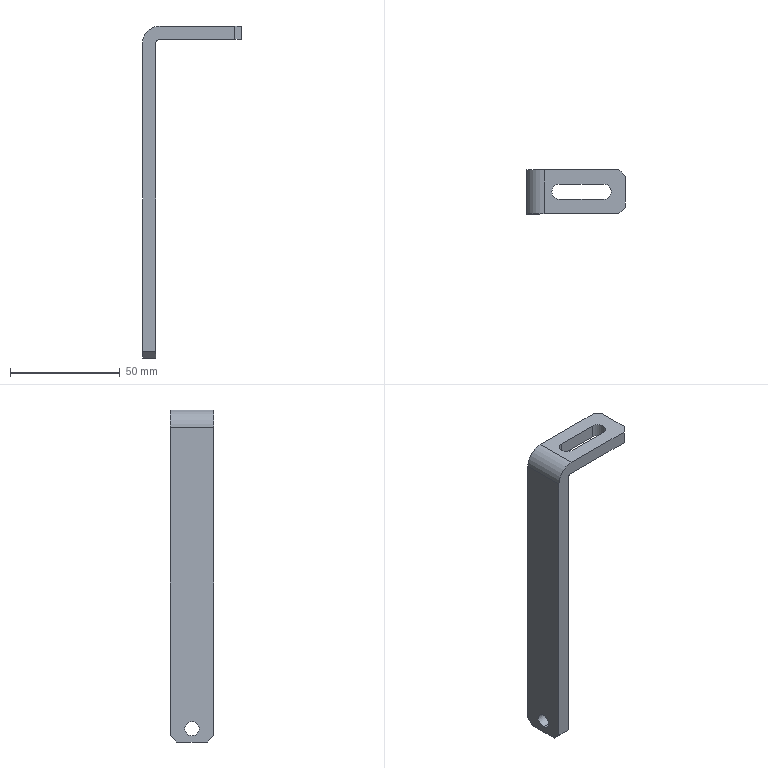Part | SolidWorks | features ICE 3, Fillet 2, Chamfer 1, Extrusion 1 | 1 solid | 21 faces | box 45 x 20 x 151 mm | volume 21164 mm3 | plane 14 | cylinder 7 | commonest cylinder face diameters 7 x3 6.5 x2 4 x1 16 x1
STEP:
#1=CARTESIAN_POINT('',(-11.,10.,75.5));
#2=VERTEX_POINT('',#1);
#3=CARTESIAN_POINT('',(-7.5,13.5,75.5));
#4=VERTEX_POINT('',#3);
#5=CARTESIAN_POINT('',(-7.5,10.,75.5));
#6=DIRECTION('',(0.,0.,-1.));
#7=DIRECTION('',(-1.,0.,0.));
#8=AXIS2_PLACEMENT_3D('',#5,#6,#7);
#9=CIRCLE('',#8,3.5);
#10=EDGE_CURVE('',#2,#4,#9,.T.);
#11=ORIENTED_EDGE('',*,*,#10,.F.);
#12=CARTESIAN_POINT('',(-11.,10.,69.5));
#13=VERTEX_POINT('',#12);
#14=CARTESIAN_POINT('',(-11.,10.,75.5));
#15=DIRECTION('',(0.,0.,-1.));
#16=VECTOR('',#15,1000.);
#17=LINE('',#14,#16);
#18=EDGE_CURVE('',#2,#13,#17,.T.);
#19=ORIENTED_EDGE('',*,*,#18,.T.);
#20=CARTESIAN_POINT('',(-7.5,13.5,69.5));
#21=VERTEX_POINT('',#20);
#22=CARTESIAN_POINT('',(-7.5,10.,69.5));
#23=DIRECTION('',(0.,0.,-1.));
#24=DIRECTION('',(-1.,0.,0.));
#25=AXIS2_PLACEMENT_3D('',#22,#23,#24);
#26=CIRCLE('',#25,3.5);
#27=EDGE_CURVE('',#13,#21,#26,.T.);
#28=ORIENTED_EDGE('',*,*,#27,.T.);
#29=CARTESIAN_POINT('',(-7.5,13.5,75.5));
#30=DIRECTION('',(0.,0.,-1.));
#31=VECTOR('',#30,1000.);
#32=LINE('',#29,#31);
#33=EDGE_CURVE('',#4,#21,#32,.T.);
#34=ORIENTED_EDGE('',*,*,#33,.F.);
#35=EDGE_LOOP('',(#11,#19,#28,#34));
#36=FACE_OUTER_BOUND('',#35,.T.);
#37=CARTESIAN_POINT('',(-7.5,10.,75.5));
#38=DIRECTION('',(0.,0.,-1.));
#39=DIRECTION('',(-1.,0.,0.));
#40=AXIS2_PLACEMENT_3D('',#37,#38,#39);
#41=CYLINDRICAL_SURFACE('',#40,3.5);
#42=ADVANCED_FACE('',(#36),#41,.F.);
#43=CARTESIAN_POINT('',(-22.5,10.,-66.25));
#44=VERTEX_POINT('',#43);
#45=CARTESIAN_POINT('',(-22.5,10.,-72.75));
#46=VERTEX_POINT('',#45);
#47=CARTESIAN_POINT('',(-22.5,10.,-69.5));
#48=DIRECTION('',(1.,0.,0.));
#49=DIRECTION('',(0.,0.,-1.));
#50=AXIS2_PLACEMENT_3D('',#47,#48,#49);
#51=CIRCLE('',#50,3.25);
#52=EDGE_CURVE('',#44,#46,#51,.T.);
#53=ORIENTED_EDGE('',*,*,#52,.F.);
#54=CARTESIAN_POINT('',(-16.5,10.,-66.25));
#55=VERTEX_POINT('',#54);
#56=CARTESIAN_POINT('',(-22.5,10.,-66.25));
#57=DIRECTION('',(1.,0.,0.));
#58=VECTOR('',#57,1000.);
#59=LINE('',#56,#58);
#60=EDGE_CURVE('',#44,#55,#59,.T.);
#61=ORIENTED_EDGE('',*,*,#60,.T.);
#62=CARTESIAN_POINT('',(-16.5,10.,-72.75));
#63=VERTEX_POINT('',#62);
#64=CARTESIAN_POINT('',(-16.5,10.,-69.5));
#65=DIRECTION('',(1.,0.,0.));
#66=DIRECTION('',(0.,0.,-1.));
#67=AXIS2_PLACEMENT_3D('',#64,#65,#66);
#68=CIRCLE('',#67,3.25);
#69=EDGE_CURVE('',#55,#63,#68,.T.);
#70=ORIENTED_EDGE('',*,*,#69,.T.);
#71=CARTESIAN_POINT('',(-22.5,10.,-72.75));
#72=DIRECTION('',(1.,0.,0.));
#73=VECTOR('',#72,1000.);
#74=LINE('',#71,#73);
#75=EDGE_CURVE('',#46,#63,#74,.T.);
#76=ORIENTED_EDGE('',*,*,#75,.F.);
#77=EDGE_LOOP('',(#53,#61,#70,#76));
#78=FACE_OUTER_BOUND('',#77,.T.);
#79=CARTESIAN_POINT('',(-22.5,10.,-69.5));
#80=DIRECTION('',(1.,0.,0.));
#81=DIRECTION('',(0.,0.,-1.));
#82=AXIS2_PLACEMENT_3D('',#79,#80,#81);
#83=CYLINDRICAL_SURFACE('',#82,3.25);
#84=ADVANCED_FACE('',(#78),#83,.F.);
#85=CARTESIAN_POINT('',(-22.5,10.,-69.5));
#86=DIRECTION('',(1.,0.,0.));
#87=DIRECTION('',(0.,0.,-1.));
#88=AXIS2_PLACEMENT_3D('',#85,#86,#87);
#89=CIRCLE('',#88,3.25);
#90=EDGE_CURVE('',#46,#44,#89,.T.);
#91=ORIENTED_EDGE('',*,*,#90,.T.);
#92=ORIENTED_EDGE('',*,*,#52,.T.);
#93=EDGE_LOOP('',(#91,#92));
#94=FACE_BOUND('',#93,.T.);
#95=CARTESIAN_POINT('',(-22.5,0.,-72.5));
#96=VERTEX_POINT('',#95);
#97=CARTESIAN_POINT('',(-22.5,0.,67.5));
#98=VERTEX_POINT('',#97);
#99=CARTESIAN_POINT('',(-22.5,0.,75.5));
#100=DIRECTION('',(0.,0.,1.));
#101=VECTOR('',#100,1000.);
#102=LINE('',#99,#101);
#103=EDGE_CURVE('',#96,#98,#102,.T.);
#104=ORIENTED_EDGE('',*,*,#103,.T.);
#105=CARTESIAN_POINT('',(-22.5,20.,67.5));
#106=VERTEX_POINT('',#105);
#107=CARTESIAN_POINT('',(-22.5,20.,67.5));
#108=DIRECTION('',(0.,1.,0.));
#109=VECTOR('',#108,1000.);
#110=LINE('',#107,#109);
#111=EDGE_CURVE('',#98,#106,#110,.T.);
#112=ORIENTED_EDGE('',*,*,#111,.T.);
#113=CARTESIAN_POINT('',(-22.5,20.,-72.5));
#114=VERTEX_POINT('',#113);
#115=CARTESIAN_POINT('',(-22.5,20.,75.5));
#116=DIRECTION('',(0.,0.,1.));
#117=VECTOR('',#116,1000.);
#118=LINE('',#115,#117);
#119=EDGE_CURVE('',#114,#106,#118,.T.);
#120=ORIENTED_EDGE('',*,*,#119,.F.);
#121=CARTESIAN_POINT('',(-22.5,17.,-75.5));
#122=VERTEX_POINT('',#121);
#123=CARTESIAN_POINT('',(-22.5,20.,-72.5));
#124=DIRECTION('',(0.,-0.7071,-0.7071));
#125=VECTOR('',#124,1000.);
#126=LINE('',#123,#125);
#127=EDGE_CURVE('',#114,#122,#126,.T.);
#128=ORIENTED_EDGE('',*,*,#127,.T.);
#129=CARTESIAN_POINT('',(-22.5,3.,-75.5));
#130=VERTEX_POINT('',#129);
#131=CARTESIAN_POINT('',(-22.5,20.,-75.5));
#132=DIRECTION('',(0.,-1.,0.));
#133=VECTOR('',#132,1000.);
#134=LINE('',#131,#133);
#135=EDGE_CURVE('',#122,#130,#134,.T.);
#136=ORIENTED_EDGE('',*,*,#135,.T.);
#137=CARTESIAN_POINT('',(-22.5,3.,-75.5));
#138=DIRECTION('',(0.,-0.7071,0.7071));
#139=VECTOR('',#138,1000.);
#140=LINE('',#137,#139);
#141=EDGE_CURVE('',#130,#96,#140,.T.);
#142=ORIENTED_EDGE('',*,*,#141,.T.);
#143=EDGE_LOOP('',(#104,#112,#120,#128,#136,#142));
#144=FACE_OUTER_BOUND('',#143,.T.);
#145=CARTESIAN_POINT('',(-22.5,20.,75.5));
#146=DIRECTION('',(1.,0.,0.));
#147=DIRECTION('',(0.,0.,-1.));
#148=AXIS2_PLACEMENT_3D('',#145,#146,#147);
#149=PLANE('',#148);
#150=ADVANCED_FACE('',(#94,#144),#149,.F.);
#151=CARTESIAN_POINT('',(12.5,13.5,75.5));
#152=VERTEX_POINT('',#151);
#153=CARTESIAN_POINT('',(12.5,13.5,75.5));
#154=DIRECTION('',(1.,0.,0.));
#155=VECTOR('',#154,1000.);
#156=LINE('',#153,#155);
#157=EDGE_CURVE('',#4,#152,#156,.T.);
#158=ORIENTED_EDGE('',*,*,#157,.T.);
#159=CARTESIAN_POINT('',(12.5,6.5,75.5));
#160=VERTEX_POINT('',#159);
#161=CARTESIAN_POINT('',(12.5,10.,75.5));
#162=DIRECTION('',(0.,0.,-1.));
#163=DIRECTION('',(-1.,0.,0.));
#164=AXIS2_PLACEMENT_3D('',#161,#162,#163);
#165=CIRCLE('',#164,3.5);
#166=EDGE_CURVE('',#152,#160,#165,.T.);
#167=ORIENTED_EDGE('',*,*,#166,.T.);
#168=CARTESIAN_POINT('',(-7.5,6.5,75.5));
#169=VERTEX_POINT('',#168);
#170=CARTESIAN_POINT('',(12.5,6.5,75.5));
#171=DIRECTION('',(-1.,0.,0.));
#172=VECTOR('',#171,1000.);
#173=LINE('',#170,#172);
#174=EDGE_CURVE('',#160,#169,#173,.T.);
#175=ORIENTED_EDGE('',*,*,#174,.T.);
#176=CARTESIAN_POINT('',(-7.5,10.,75.5));
#177=DIRECTION('',(0.,0.,-1.));
#178=DIRECTION('',(-1.,0.,0.));
#179=AXIS2_PLACEMENT_3D('',#176,#177,#178);
#180=CIRCLE('',#179,3.5);
#181=EDGE_CURVE('',#169,#2,#180,.T.);
#182=ORIENTED_EDGE('',*,*,#181,.T.);
#183=ORIENTED_EDGE('',*,*,#10,.T.);
#184=EDGE_LOOP('',(#158,#167,#175,#182,#183));
#185=FACE_BOUND('',#184,.T.);
#186=CARTESIAN_POINT('',(-14.5,20.,75.5));
#187=VERTEX_POINT('',#186);
#188=CARTESIAN_POINT('',(19.5,20.,75.5));
#189=VERTEX_POINT('',#188);
#190=CARTESIAN_POINT('',(22.5,20.,75.5));
#191=DIRECTION('',(1.,0.,0.));
#192=VECTOR('',#191,1000.);
#193=LINE('',#190,#192);
#194=EDGE_CURVE('',#187,#189,#193,.T.);
#195=ORIENTED_EDGE('',*,*,#194,.F.);
#196=CARTESIAN_POINT('',(-14.5,0.,75.5));
#197=VERTEX_POINT('',#196);
#198=CARTESIAN_POINT('',(-14.5,20.,75.5));
#199=DIRECTION('',(0.,-1.,0.));
#200=VECTOR('',#199,1000.);
#201=LINE('',#198,#200);
#202=EDGE_CURVE('',#187,#197,#201,.T.);
#203=ORIENTED_EDGE('',*,*,#202,.T.);
#204=CARTESIAN_POINT('',(19.5,0.,75.5));
#205=VERTEX_POINT('',#204);
#206=CARTESIAN_POINT('',(22.5,0.,75.5));
#207=DIRECTION('',(1.,0.,0.));
#208=VECTOR('',#207,1000.);
#209=LINE('',#206,#208);
#210=EDGE_CURVE('',#197,#205,#209,.T.);
#211=ORIENTED_EDGE('',*,*,#210,.T.);
#212=CARTESIAN_POINT('',(22.5,3.,75.5));
#213=VERTEX_POINT('',#212);
#214=CARTESIAN_POINT('',(22.5,3.,75.5));
#215=DIRECTION('',(0.7071,0.7071,0.));
#216=VECTOR('',#215,1000.);
#217=LINE('',#214,#216);
#218=EDGE_CURVE('',#205,#213,#217,.T.);
#219=ORIENTED_EDGE('',*,*,#218,.T.);
#220=CARTESIAN_POINT('',(22.5,17.,75.5));
#221=VERTEX_POINT('',#220);
#222=CARTESIAN_POINT('',(22.5,20.,75.5));
#223=DIRECTION('',(0.,-1.,0.));
#224=VECTOR('',#223,1000.);
#225=LINE('',#222,#224);
#226=EDGE_CURVE('',#221,#213,#225,.T.);
#227=ORIENTED_EDGE('',*,*,#226,.F.);
#228=CARTESIAN_POINT('',(19.5,20.,75.5));
#229=DIRECTION('',(-0.7071,0.7071,0.));
#230=VECTOR('',#229,1000.);
#231=LINE('',#228,#230);
#232=EDGE_CURVE('',#221,#189,#231,.T.);
#233=ORIENTED_EDGE('',*,*,#232,.T.);
#234=EDGE_LOOP('',(#195,#203,#211,#219,#227,#233));
#235=FACE_OUTER_BOUND('',#234,.T.);
#236=CARTESIAN_POINT('',(22.5,20.,75.5));
#237=DIRECTION('',(0.,0.,-1.));
#238=DIRECTION('',(-1.,0.,0.));
#239=AXIS2_PLACEMENT_3D('',#236,#237,#238);
#240=PLANE('',#239);
#241=ADVANCED_FACE('',(#185,#235),#240,.F.);
#242=ORIENTED_EDGE('',*,*,#226,.T.);
#243=CARTESIAN_POINT('',(22.5,3.,69.5));
#244=VERTEX_POINT('',#243);
#245=CARTESIAN_POINT('',(22.5,3.,75.5));
#246=DIRECTION('',(0.,0.,-1.));
#247=VECTOR('',#246,1000.);
#248=LINE('',#245,#247);
#249=EDGE_CURVE('',#213,#244,#248,.T.);
#250=ORIENTED_EDGE('',*,*,#249,.T.);
#251=CARTESIAN_POINT('',(22.5,17.,69.5));
#252=VERTEX_POINT('',#251);
#253=CARTESIAN_POINT('',(22.5,0.,69.5));
#254=DIRECTION('',(0.,1.,0.));
#255=VECTOR('',#254,1000.);
#256=LINE('',#253,#255);
#257=EDGE_CURVE('',#244,#252,#256,.T.);
#258=ORIENTED_EDGE('',*,*,#257,.T.);
#259=CARTESIAN_POINT('',(22.5,17.,75.5));
#260=DIRECTION('',(0.,0.,1.));
#261=VECTOR('',#260,1000.);
#262=LINE('',#259,#261);
#263=EDGE_CURVE('',#252,#221,#262,.T.);
#264=ORIENTED_EDGE('',*,*,#263,.T.);
#265=EDGE_LOOP('',(#242,#250,#258,#264));
#266=FACE_OUTER_BOUND('',#265,.T.);
#267=CARTESIAN_POINT('',(22.5,20.,75.5));
#268=DIRECTION('',(-1.,0.,0.));
#269=DIRECTION('',(0.,0.,1.));
#270=AXIS2_PLACEMENT_3D('',#267,#268,#269);
#271=PLANE('',#270);
#272=ADVANCED_FACE('',(#266),#271,.F.);
#273=CARTESIAN_POINT('',(-16.5,3.,-75.5));
#274=VERTEX_POINT('',#273);
#275=CARTESIAN_POINT('',(-16.5,17.,-75.5));
#276=VERTEX_POINT('',#275);
#277=CARTESIAN_POINT('',(-16.5,0.,-75.5));
#278=DIRECTION('',(0.,1.,0.));
#279=VECTOR('',#278,1000.);
#280=LINE('',#277,#279);
#281=EDGE_CURVE('',#274,#276,#280,.T.);
#282=ORIENTED_EDGE('',*,*,#281,.F.);
#283=CARTESIAN_POINT('',(22.5,3.,-75.5));
#284=DIRECTION('',(-1.,0.,0.));
#285=VECTOR('',#284,1000.);
#286=LINE('',#283,#285);
#287=EDGE_CURVE('',#274,#130,#286,.T.);
#288=ORIENTED_EDGE('',*,*,#287,.T.);
#289=ORIENTED_EDGE('',*,*,#135,.F.);
#290=CARTESIAN_POINT('',(-16.5,17.,-75.5));
#291=DIRECTION('',(1.,0.,0.));
#292=VECTOR('',#291,1000.);
#293=LINE('',#290,#292);
#294=EDGE_CURVE('',#122,#276,#293,.T.);
#295=ORIENTED_EDGE('',*,*,#294,.T.);
#296=EDGE_LOOP('',(#282,#288,#289,#295));
#297=FACE_OUTER_BOUND('',#296,.T.);
#298=CARTESIAN_POINT('',(22.5,20.,-75.5));
#299=DIRECTION('',(0.,0.,1.));
#300=DIRECTION('',(1.,0.,0.));
#301=AXIS2_PLACEMENT_3D('',#298,#299,#300);
#302=PLANE('',#301);
#303=ADVANCED_FACE('',(#297),#302,.F.);
#304=ORIENTED_EDGE('',*,*,#119,.T.);
#305=CARTESIAN_POINT('',(-14.5,20.,67.5));
#306=DIRECTION('',(0.,1.,0.));
#307=DIRECTION('',(0.,0.,1.));
#308=AXIS2_PLACEMENT_3D('',#305,#306,#307);
#309=CIRCLE('',#308,8.);
#310=EDGE_CURVE('',#106,#187,#309,.T.);
#311=ORIENTED_EDGE('',*,*,#310,.T.);
#312=ORIENTED_EDGE('',*,*,#194,.T.);
#313=CARTESIAN_POINT('',(19.5,20.,69.5));
#314=VERTEX_POINT('',#313);
#315=CARTESIAN_POINT('',(19.5,20.,69.5));
#316=DIRECTION('',(0.,0.,-1.));
#317=VECTOR('',#316,1000.);
#318=LINE('',#315,#317);
#319=EDGE_CURVE('',#189,#314,#318,.T.);
#320=ORIENTED_EDGE('',*,*,#319,.T.);
#321=CARTESIAN_POINT('',(-14.5,20.,69.5));
#322=VERTEX_POINT('',#321);
#323=CARTESIAN_POINT('',(22.5,20.,69.5));
#324=DIRECTION('',(1.,0.,0.));
#325=VECTOR('',#324,1000.);
#326=LINE('',#323,#325);
#327=EDGE_CURVE('',#322,#314,#326,.T.);
#328=ORIENTED_EDGE('',*,*,#327,.F.);
#329=CARTESIAN_POINT('',(-16.5,20.,67.5));
#330=VERTEX_POINT('',#329);
#331=CARTESIAN_POINT('',(-14.5,20.,67.5));
#332=DIRECTION('',(0.,-1.,0.));
#333=DIRECTION('',(0.,0.,1.));
#334=AXIS2_PLACEMENT_3D('',#331,#332,#333);
#335=CIRCLE('',#334,2.);
#336=EDGE_CURVE('',#322,#330,#335,.T.);
#337=ORIENTED_EDGE('',*,*,#336,.T.);
#338=CARTESIAN_POINT('',(-16.5,20.,-72.5));
#339=VERTEX_POINT('',#338);
#340=CARTESIAN_POINT('',(-16.5,20.,-75.5));
#341=DIRECTION('',(0.,0.,1.));
#342=VECTOR('',#341,1000.);
#343=LINE('',#340,#342);
#344=EDGE_CURVE('',#339,#330,#343,.T.);
#345=ORIENTED_EDGE('',*,*,#344,.F.);
#346=CARTESIAN_POINT('',(-22.5,20.,-72.5));
#347=DIRECTION('',(-1.,0.,0.));
#348=VECTOR('',#347,1000.);
#349=LINE('',#346,#348);
#350=EDGE_CURVE('',#339,#114,#349,.T.);
#351=ORIENTED_EDGE('',*,*,#350,.T.);
#352=EDGE_LOOP('',(#304,#311,#312,#320,#328,#337,#345,#351));
#353=FACE_OUTER_BOUND('',#352,.T.);
#354=CARTESIAN_POINT('',(-22.5,20.,-75.5));
#355=DIRECTION('',(0.,1.,0.));
#356=DIRECTION('',(0.,0.,1.));
#357=AXIS2_PLACEMENT_3D('',#354,#355,#356);
#358=PLANE('',#357);
#359=ADVANCED_FACE('',(#353),#358,.T.);
#360=ORIENTED_EDGE('',*,*,#210,.F.);
#361=CARTESIAN_POINT('',(-14.5,0.,67.5));
#362=DIRECTION('',(0.,-1.,0.));
#363=DIRECTION('',(0.,0.,1.));
#364=AXIS2_PLACEMENT_3D('',#361,#362,#363);
#365=CIRCLE('',#364,8.);
#366=EDGE_CURVE('',#197,#98,#365,.T.);
#367=ORIENTED_EDGE('',*,*,#366,.T.);
#368=ORIENTED_EDGE('',*,*,#103,.F.);
#369=CARTESIAN_POINT('',(-16.5,0.,-72.5));
#370=VERTEX_POINT('',#369);
#371=CARTESIAN_POINT('',(-22.5,0.,-72.5));
#372=DIRECTION('',(1.,0.,0.));
#373=VECTOR('',#372,1000.);
#374=LINE('',#371,#373);
#375=EDGE_CURVE('',#96,#370,#374,.T.);
#376=ORIENTED_EDGE('',*,*,#375,.T.);
#377=CARTESIAN_POINT('',(-16.5,0.,67.5));
#378=VERTEX_POINT('',#377);
#379=CARTESIAN_POINT('',(-16.5,0.,-75.5));
#380=DIRECTION('',(0.,0.,1.));
#381=VECTOR('',#380,1000.);
#382=LINE('',#379,#381);
#383=EDGE_CURVE('',#370,#378,#382,.T.);
#384=ORIENTED_EDGE('',*,*,#383,.T.);
#385=CARTESIAN_POINT('',(-14.5,0.,69.5));
#386=VERTEX_POINT('',#385);
#387=CARTESIAN_POINT('',(-14.5,0.,67.5));
#388=DIRECTION('',(0.,1.,0.));
#389=DIRECTION('',(0.,0.,1.));
#390=AXIS2_PLACEMENT_3D('',#387,#388,#389);
#391=CIRCLE('',#390,2.);
#392=EDGE_CURVE('',#378,#386,#391,.T.);
#393=ORIENTED_EDGE('',*,*,#392,.T.);
#394=CARTESIAN_POINT('',(19.5,0.,69.5));
#395=VERTEX_POINT('',#394);
#396=CARTESIAN_POINT('',(22.5,0.,69.5));
#397=DIRECTION('',(1.,0.,0.));
#398=VECTOR('',#397,1000.);
#399=LINE('',#396,#398);
#400=EDGE_CURVE('',#386,#395,#399,.T.);
#401=ORIENTED_EDGE('',*,*,#400,.T.);
#402=CARTESIAN_POINT('',(19.5,0.,-75.5));
#403=DIRECTION('',(0.,0.,1.));
#404=VECTOR('',#403,1000.);
#405=LINE('',#402,#404);
#406=EDGE_CURVE('',#395,#205,#405,.T.);
#407=ORIENTED_EDGE('',*,*,#406,.T.);
#408=EDGE_LOOP('',(#360,#367,#368,#376,#384,#393,#401,#407));
#409=FACE_OUTER_BOUND('',#408,.T.);
#410=CARTESIAN_POINT('',(-22.5,0.,-75.5));
#411=DIRECTION('',(0.,1.,0.));
#412=DIRECTION('',(0.,0.,1.));
#413=AXIS2_PLACEMENT_3D('',#410,#411,#412);
#414=PLANE('',#413);
#415=ADVANCED_FACE('',(#409),#414,.F.);
#416=CARTESIAN_POINT('',(12.5,6.5,69.5));
#417=VERTEX_POINT('',#416);
#418=CARTESIAN_POINT('',(-7.5,6.5,69.5));
#419=VERTEX_POINT('',#418);
#420=CARTESIAN_POINT('',(12.5,6.5,69.5));
#421=DIRECTION('',(-1.,0.,0.));
#422=VECTOR('',#421,1000.);
#423=LINE('',#420,#422);
#424=EDGE_CURVE('',#417,#419,#423,.T.);
#425=ORIENTED_EDGE('',*,*,#424,.F.);
#426=CARTESIAN_POINT('',(12.5,13.5,69.5));
#427=VERTEX_POINT('',#426);
#428=CARTESIAN_POINT('',(12.5,10.,69.5));
#429=DIRECTION('',(0.,0.,-1.));
#430=DIRECTION('',(-1.,0.,0.));
#431=AXIS2_PLACEMENT_3D('',#428,#429,#430);
#432=CIRCLE('',#431,3.5);
#433=EDGE_CURVE('',#427,#417,#432,.T.);
#434=ORIENTED_EDGE('',*,*,#433,.F.);
#435=CARTESIAN_POINT('',(12.5,13.5,69.5));
#436=DIRECTION('',(1.,0.,0.));
#437=VECTOR('',#436,1000.);
#438=LINE('',#435,#437);
#439=EDGE_CURVE('',#21,#427,#438,.T.);
#440=ORIENTED_EDGE('',*,*,#439,.F.);
#441=ORIENTED_EDGE('',*,*,#27,.F.);
#442=CARTESIAN_POINT('',(-7.5,10.,69.5));
#443=DIRECTION('',(0.,0.,-1.));
#444=DIRECTION('',(-1.,0.,0.));
#445=AXIS2_PLACEMENT_3D('',#442,#443,#444);
#446=CIRCLE('',#445,3.5);
#447=EDGE_CURVE('',#419,#13,#446,.T.);
#448=ORIENTED_EDGE('',*,*,#447,.F.);
#449=EDGE_LOOP('',(#425,#434,#440,#441,#448));
#450=FACE_BOUND('',#449,.T.);
#451=ORIENTED_EDGE('',*,*,#400,.F.);
#452=CARTESIAN_POINT('',(-14.5,20.,69.5));
#453=DIRECTION('',(0.,1.,0.));
#454=VECTOR('',#453,1000.);
#455=LINE('',#452,#454);
#456=EDGE_CURVE('',#386,#322,#455,.T.);
#457=ORIENTED_EDGE('',*,*,#456,.T.);
#458=ORIENTED_EDGE('',*,*,#327,.T.);
#459=CARTESIAN_POINT('',(19.5,20.,69.5));
#460=DIRECTION('',(0.7071,-0.7071,0.));
#461=VECTOR('',#460,1000.);
#462=LINE('',#459,#461);
#463=EDGE_CURVE('',#314,#252,#462,.T.);
#464=ORIENTED_EDGE('',*,*,#463,.T.);
#465=ORIENTED_EDGE('',*,*,#257,.F.);
#466=CARTESIAN_POINT('',(22.5,3.,69.5));
#467=DIRECTION('',(-0.7071,-0.7071,0.));
#468=VECTOR('',#467,1000.);
#469=LINE('',#466,#468);
#470=EDGE_CURVE('',#244,#395,#469,.T.);
#471=ORIENTED_EDGE('',*,*,#470,.T.);
#472=EDGE_LOOP('',(#451,#457,#458,#464,#465,#471));
#473=FACE_OUTER_BOUND('',#472,.T.);
#474=CARTESIAN_POINT('',(22.5,0.,69.5));
#475=DIRECTION('',(0.,0.,1.));
#476=DIRECTION('',(1.,0.,0.));
#477=AXIS2_PLACEMENT_3D('',#474,#475,#476);
#478=PLANE('',#477);
#479=ADVANCED_FACE('',(#450,#473),#478,.F.);
#480=CARTESIAN_POINT('',(-16.5,10.,-69.5));
#481=DIRECTION('',(1.,0.,0.));
#482=DIRECTION('',(0.,0.,-1.));
#483=AXIS2_PLACEMENT_3D('',#480,#481,#482);
#484=CIRCLE('',#483,3.25);
#485=EDGE_CURVE('',#63,#55,#484,.T.);
#486=ORIENTED_EDGE('',*,*,#485,.F.);
#487=ORIENTED_EDGE('',*,*,#69,.F.);
#488=EDGE_LOOP('',(#486,#487));
#489=FACE_BOUND('',#488,.T.);
#490=ORIENTED_EDGE('',*,*,#344,.T.);
#491=CARTESIAN_POINT('',(-16.5,0.,67.5));
#492=DIRECTION('',(0.,-1.,0.));
#493=VECTOR('',#492,1000.);
#494=LINE('',#491,#493);
#495=EDGE_CURVE('',#330,#378,#494,.T.);
#496=ORIENTED_EDGE('',*,*,#495,.T.);
#497=ORIENTED_EDGE('',*,*,#383,.F.);
#498=CARTESIAN_POINT('',(-16.5,3.,-75.5));
#499=DIRECTION('',(0.,0.7071,-0.7071));
#500=VECTOR('',#499,1000.);
#501=LINE('',#498,#500);
#502=EDGE_CURVE('',#370,#274,#501,.T.);
#503=ORIENTED_EDGE('',*,*,#502,.T.);
#504=ORIENTED_EDGE('',*,*,#281,.T.);
#505=CARTESIAN_POINT('',(-16.5,20.,-72.5));
#506=DIRECTION('',(0.,0.7071,0.7071));
#507=VECTOR('',#506,1000.);
#508=LINE('',#505,#507);
#509=EDGE_CURVE('',#276,#339,#508,.T.);
#510=ORIENTED_EDGE('',*,*,#509,.T.);
#511=EDGE_LOOP('',(#490,#496,#497,#503,#504,#510));
#512=FACE_OUTER_BOUND('',#511,.T.);
#513=CARTESIAN_POINT('',(-16.5,0.,-75.5));
#514=DIRECTION('',(-1.,0.,0.));
#515=DIRECTION('',(0.,0.,1.));
#516=AXIS2_PLACEMENT_3D('',#513,#514,#515);
#517=PLANE('',#516);
#518=ADVANCED_FACE('',(#489,#512),#517,.F.);
#519=ORIENTED_EDGE('',*,*,#60,.F.);
#520=ORIENTED_EDGE('',*,*,#90,.F.);
#521=ORIENTED_EDGE('',*,*,#75,.T.);
#522=ORIENTED_EDGE('',*,*,#485,.T.);
#523=EDGE_LOOP('',(#519,#520,#521,#522));
#524=FACE_OUTER_BOUND('',#523,.T.);
#525=CARTESIAN_POINT('',(-22.5,10.,-69.5));
#526=DIRECTION('',(1.,0.,0.));
#527=DIRECTION('',(0.,0.,-1.));
#528=AXIS2_PLACEMENT_3D('',#525,#526,#527);
#529=CYLINDRICAL_SURFACE('',#528,3.25);
#530=ADVANCED_FACE('',(#524),#529,.F.);
#531=ORIENTED_EDGE('',*,*,#433,.T.);
#532=CARTESIAN_POINT('',(12.5,6.5,75.5));
#533=DIRECTION('',(0.,0.,-1.));
#534=VECTOR('',#533,1000.);
#535=LINE('',#532,#534);
#536=EDGE_CURVE('',#160,#417,#535,.T.);
#537=ORIENTED_EDGE('',*,*,#536,.F.);
#538=ORIENTED_EDGE('',*,*,#166,.F.);
#539=CARTESIAN_POINT('',(12.5,13.5,75.5));
#540=DIRECTION('',(0.,0.,-1.));
#541=VECTOR('',#540,1000.);
#542=LINE('',#539,#541);
#543=EDGE_CURVE('',#152,#427,#542,.T.);
#544=ORIENTED_EDGE('',*,*,#543,.T.);
#545=EDGE_LOOP('',(#531,#537,#538,#544));
#546=FACE_OUTER_BOUND('',#545,.T.);
#547=CARTESIAN_POINT('',(12.5,10.,75.5));
#548=DIRECTION('',(0.,0.,-1.));
#549=DIRECTION('',(-1.,0.,0.));
#550=AXIS2_PLACEMENT_3D('',#547,#548,#549);
#551=CYLINDRICAL_SURFACE('',#550,3.5);
#552=ADVANCED_FACE('',(#546),#551,.F.);
#553=ORIENTED_EDGE('',*,*,#439,.T.);
#554=ORIENTED_EDGE('',*,*,#543,.F.);
#555=ORIENTED_EDGE('',*,*,#157,.F.);
#556=ORIENTED_EDGE('',*,*,#33,.T.);
#557=EDGE_LOOP('',(#553,#554,#555,#556));
#558=FACE_OUTER_BOUND('',#557,.T.);
#559=CARTESIAN_POINT('',(12.5,13.5,75.5));
#560=DIRECTION('',(0.,1.,0.));
#561=DIRECTION('',(0.,0.,1.));
#562=AXIS2_PLACEMENT_3D('',#559,#560,#561);
#563=PLANE('',#562);
#564=ADVANCED_FACE('',(#558),#563,.F.);
#565=ORIENTED_EDGE('',*,*,#18,.F.);
#566=ORIENTED_EDGE('',*,*,#181,.F.);
#567=CARTESIAN_POINT('',(-7.5,6.5,75.5));
#568=DIRECTION('',(0.,0.,-1.));
#569=VECTOR('',#568,1000.);
#570=LINE('',#567,#569);
#571=EDGE_CURVE('',#169,#419,#570,.T.);
#572=ORIENTED_EDGE('',*,*,#571,.T.);
#573=ORIENTED_EDGE('',*,*,#447,.T.);
#574=EDGE_LOOP('',(#565,#566,#572,#573));
#575=FACE_OUTER_BOUND('',#574,.T.);
#576=CARTESIAN_POINT('',(-7.5,10.,75.5));
#577=DIRECTION('',(0.,0.,-1.));
#578=DIRECTION('',(-1.,0.,0.));
#579=AXIS2_PLACEMENT_3D('',#576,#577,#578);
#580=CYLINDRICAL_SURFACE('',#579,3.5);
#581=ADVANCED_FACE('',(#575),#580,.F.);
#582=ORIENTED_EDGE('',*,*,#424,.T.);
#583=ORIENTED_EDGE('',*,*,#571,.F.);
#584=ORIENTED_EDGE('',*,*,#174,.F.);
#585=ORIENTED_EDGE('',*,*,#536,.T.);
#586=EDGE_LOOP('',(#582,#583,#584,#585));
#587=FACE_OUTER_BOUND('',#586,.T.);
#588=CARTESIAN_POINT('',(12.5,6.5,75.5));
#589=DIRECTION('',(0.,-1.,0.));
#590=DIRECTION('',(0.,0.,-1.));
#591=AXIS2_PLACEMENT_3D('',#588,#589,#590);
#592=PLANE('',#591);
#593=ADVANCED_FACE('',(#587),#592,.F.);
#594=ORIENTED_EDGE('',*,*,#218,.F.);
#595=ORIENTED_EDGE('',*,*,#406,.F.);
#596=ORIENTED_EDGE('',*,*,#470,.F.);
#597=ORIENTED_EDGE('',*,*,#249,.F.);
#598=EDGE_LOOP('',(#594,#595,#596,#597));
#599=FACE_OUTER_BOUND('',#598,.T.);
#600=CARTESIAN_POINT('',(22.5,3.,75.5));
#601=DIRECTION('',(-0.7071,0.7071,0.));
#602=DIRECTION('',(-0.7071,-0.7071,0.));
#603=AXIS2_PLACEMENT_3D('',#600,#601,#602);
#604=PLANE('',#603);
#605=ADVANCED_FACE('',(#599),#604,.F.);
#606=ORIENTED_EDGE('',*,*,#232,.F.);
#607=ORIENTED_EDGE('',*,*,#263,.F.);
#608=ORIENTED_EDGE('',*,*,#463,.F.);
#609=ORIENTED_EDGE('',*,*,#319,.F.);
#610=EDGE_LOOP('',(#606,#607,#608,#609));
#611=FACE_OUTER_BOUND('',#610,.T.);
#612=CARTESIAN_POINT('',(19.5,20.,-75.5));
#613=DIRECTION('',(0.7071,0.7071,0.));
#614=DIRECTION('',(-0.7071,0.7071,0.));
#615=AXIS2_PLACEMENT_3D('',#612,#613,#614);
#616=PLANE('',#615);
#617=ADVANCED_FACE('',(#611),#616,.T.);
#618=ORIENTED_EDGE('',*,*,#502,.F.);
#619=ORIENTED_EDGE('',*,*,#375,.F.);
#620=ORIENTED_EDGE('',*,*,#141,.F.);
#621=ORIENTED_EDGE('',*,*,#287,.F.);
#622=EDGE_LOOP('',(#618,#619,#620,#621));
#623=FACE_OUTER_BOUND('',#622,.T.);
#624=CARTESIAN_POINT('',(22.5,3.,-75.5));
#625=DIRECTION('',(0.,0.7071,0.7071));
#626=DIRECTION('',(0.,-0.7071,0.7071));
#627=AXIS2_PLACEMENT_3D('',#624,#625,#626);
#628=PLANE('',#627);
#629=ADVANCED_FACE('',(#623),#628,.F.);
#630=ORIENTED_EDGE('',*,*,#509,.F.);
#631=ORIENTED_EDGE('',*,*,#294,.F.);
#632=ORIENTED_EDGE('',*,*,#127,.F.);
#633=ORIENTED_EDGE('',*,*,#350,.F.);
#634=EDGE_LOOP('',(#630,#631,#632,#633));
#635=FACE_OUTER_BOUND('',#634,.T.);
#636=CARTESIAN_POINT('',(-22.5,20.,-72.5));
#637=DIRECTION('',(0.,0.7071,-0.7071));
#638=DIRECTION('',(0.,0.7071,0.7071));
#639=AXIS2_PLACEMENT_3D('',#636,#637,#638);
#640=PLANE('',#639);
#641=ADVANCED_FACE('',(#635),#640,.T.);
#642=ORIENTED_EDGE('',*,*,#392,.F.);
#643=ORIENTED_EDGE('',*,*,#495,.F.);
#644=ORIENTED_EDGE('',*,*,#336,.F.);
#645=ORIENTED_EDGE('',*,*,#456,.F.);
#646=EDGE_LOOP('',(#642,#643,#644,#645));
#647=FACE_OUTER_BOUND('',#646,.T.);
#648=CARTESIAN_POINT('',(-14.5,0.,67.5));
#649=DIRECTION('',(0.,-1.,0.));
#650=DIRECTION('',(0.,0.,-1.));
#651=AXIS2_PLACEMENT_3D('',#648,#649,#650);
#652=CYLINDRICAL_SURFACE('',#651,2.);
#653=ADVANCED_FACE('',(#647),#652,.F.);
#654=ORIENTED_EDGE('',*,*,#310,.F.);
#655=ORIENTED_EDGE('',*,*,#111,.F.);
#656=ORIENTED_EDGE('',*,*,#366,.F.);
#657=ORIENTED_EDGE('',*,*,#202,.F.);
#658=EDGE_LOOP('',(#654,#655,#656,#657));
#659=FACE_OUTER_BOUND('',#658,.T.);
#660=CARTESIAN_POINT('',(-14.5,20.,67.5));
#661=DIRECTION('',(0.,-1.,0.));
#662=DIRECTION('',(0.,0.,-1.));
#663=AXIS2_PLACEMENT_3D('',#660,#661,#662);
#664=CYLINDRICAL_SURFACE('',#663,8.);
#665=ADVANCED_FACE('',(#659),#664,.T.);
#666=CLOSED_SHELL('',(#42,#84,#150,#241,#272,#303,#359,#415,#479,#518,#530,#552,#564,#581,#593,#605,#617,#629,#641,#653,#665));
#667=MANIFOLD_SOLID_BREP('',#666);
#668=CARTESIAN_POINT('',(0.,0.,0.));
#669=DIRECTION('',(0.,0.,1.));
#670=DIRECTION('',(1.,0.,0.));
#671=AXIS2_PLACEMENT_3D('',#668,#669,#670);
#672=(LENGTH_UNIT()NAMED_UNIT(*)SI_UNIT(.MILLI.,.METRE.));
#673=UNCERTAINTY_MEASURE_WITH_UNIT(LENGTH_MEASURE(0.00001),#672,'','');
#674=(NAMED_UNIT(*)PLANE_ANGLE_UNIT()SI_UNIT($,.RADIAN.));
#675=(NAMED_UNIT(*)SI_UNIT($,.STERADIAN.)SOLID_ANGLE_UNIT());
#676=(GEOMETRIC_REPRESENTATION_CONTEXT(3)GLOBAL_UNCERTAINTY_ASSIGNED_CONTEXT((#673))GLOBAL_UNIT_ASSIGNED_CONTEXT((#672,#674,#675))REPRESENTATION_CONTEXT('',''));
#677=ADVANCED_BREP_SHAPE_REPRESENTATION('',(#667,#671),#676);